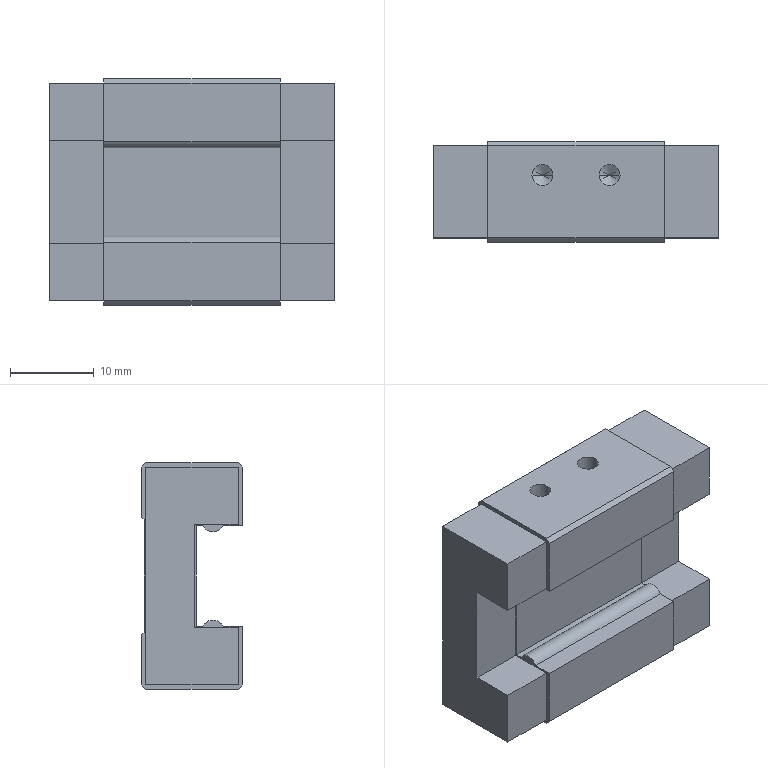Part | NX | 1 solid | 73 faces | box 34 x 12 x 27 mm | volume 8069 mm3 | plane 38 | cylinder 19 | cone 16 | commonest cylinder face diameters 2.5 x16 2.7 x3